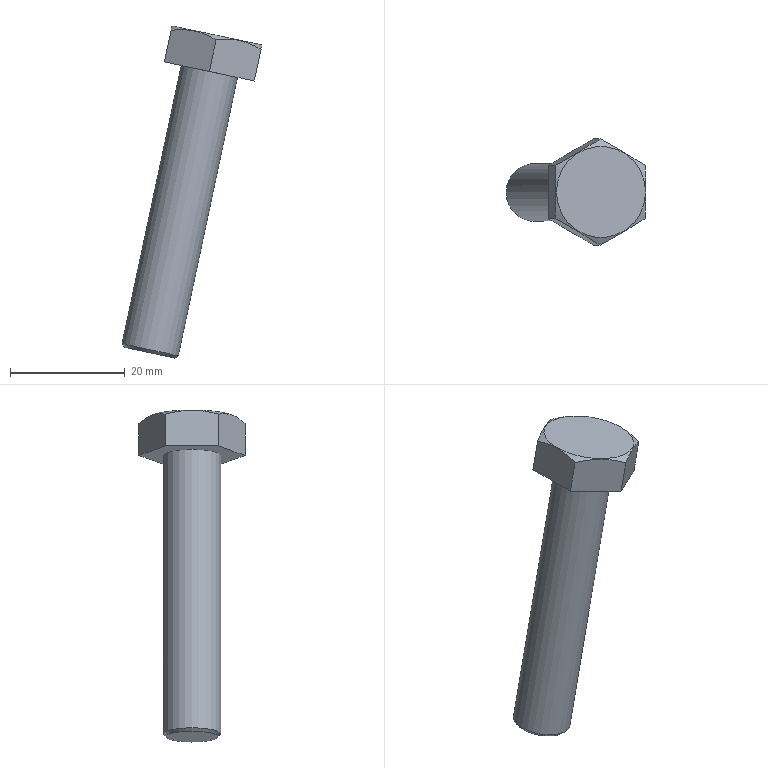Part | STEP file | 8901-M1050B (bolt M12×50) | 1 solid | 12 faces | box 24.329 x 18.475 x 57.75 mm | volume 5337 mm3 | plane 9 | cone 2 | cylinder 1 | commonest cylinder face diameters 10 x1
STEP:
#1=CARTESIAN_POINT('',(0.,0.,0.));
#2=DIRECTION('',(0.,0.,1.));
#3=DIRECTION('',(1.,0.,0.));
#4=AXIS2_PLACEMENT_3D('',#1,#2,#3);
#5=CARTESIAN_POINT('',(1860.531,-39.5,-396.681));
#6=VERTEX_POINT('',#5);
#7=CARTESIAN_POINT('',(1865.421,-39.5,-397.721));
#8=DIRECTION('',(0.2079,0.,0.9781));
#9=DIRECTION('',(-0.9781,0.,0.2079));
#10=AXIS2_PLACEMENT_3D('',#7,#8,#9);
#11=CIRCLE('',#10,5.);
#12=CARTESIAN_POINT('',(1865.421,-39.5,-397.721));
#13=DIRECTION('',(0.2079,0.,0.9781));
#14=DIRECTION('',(-0.9781,0.,0.2079));
#15=AXIS2_PLACEMENT_3D('',#12,#13,#14);
#16=CONICAL_SURFACE('',#15,5.,0.7854);
#17=CARTESIAN_POINT('',(0.,0.));
#18=DIRECTION('',(1.,0.));
#19=VECTOR('',#18,1.);
#20=LINE('',#17,#19);
#21=(GEOMETRIC_REPRESENTATION_CONTEXT(2)PARAMETRIC_REPRESENTATION_CONTEXT()REPRESENTATION_CONTEXT('',''));
#22=DEFINITIONAL_REPRESENTATION('',(#20),#21);
#23=PCURVE('',#16,#22);
#24=CARTESIAN_POINT('',(1875.713,-39.5,-349.303));
#25=DIRECTION('',(-0.2079,0.,-0.9781));
#26=DIRECTION('',(0.9781,0.,-0.2079));
#27=AXIS2_PLACEMENT_3D('',#24,#25,#26);
#28=CYLINDRICAL_SURFACE('',#27,5.);
#29=CARTESIAN_POINT('',(9.425,49.5));
#30=DIRECTION('',(-1.,0.));
#31=VECTOR('',#30,1.);
#32=LINE('',#29,#31);
#33=(GEOMETRIC_REPRESENTATION_CONTEXT(2)PARAMETRIC_REPRESENTATION_CONTEXT()REPRESENTATION_CONTEXT('',''));
#34=DEFINITIONAL_REPRESENTATION('',(#32),#33);
#35=PCURVE('',#28,#34);
#36=SURFACE_CURVE('',#11,(#23,#35),.PCURVE_S1.);
#37=EDGE_CURVE('',#6,#6,#36,.T.);
#38=ORIENTED_EDGE('',*,*,#37,.F.);
#39=CARTESIAN_POINT('',(1860.916,-39.5,-397.274));
#40=VERTEX_POINT('',#39);
#41=CARTESIAN_POINT('',(1860.916,-39.5,-397.274));
#42=CARTESIAN_POINT('',(1860.531,-39.5,-396.681));
#43=B_SPLINE_CURVE_WITH_KNOTS('',1,(#41,#42),.UNSPECIFIED.,.F.,.F.,(2,2),(-0.7071,0.),.PIECEWISE_BEZIER_KNOTS.);
#44=CARTESIAN_POINT('',(0.,0.));
#45=DIRECTION('',(0.,1.));
#46=VECTOR('',#45,1.);
#47=LINE('',#44,#46);
#48=(GEOMETRIC_REPRESENTATION_CONTEXT(2)PARAMETRIC_REPRESENTATION_CONTEXT()REPRESENTATION_CONTEXT('',''));
#49=DEFINITIONAL_REPRESENTATION('',(#47),#48);
#50=PCURVE('',#16,#49);
#51=CARTESIAN_POINT('',(6.283,0.));
#52=DIRECTION('',(0.,1.));
#53=VECTOR('',#52,1.);
#54=LINE('',#51,#53);
#55=(GEOMETRIC_REPRESENTATION_CONTEXT(2)PARAMETRIC_REPRESENTATION_CONTEXT()REPRESENTATION_CONTEXT('',''));
#56=DEFINITIONAL_REPRESENTATION('',(#54),#55);
#57=PCURVE('',#16,#56);
#58=SEAM_CURVE('',#43,(#50,#57),.PCURVE_S1.);
#59=EDGE_CURVE('',#40,#6,#58,.T.);
#60=ORIENTED_EDGE('',*,*,#59,.F.);
#61=CARTESIAN_POINT('',(1865.317,-39.5,-398.21));
#62=DIRECTION('',(-0.2079,0.,-0.9781));
#63=DIRECTION('',(-0.9781,0.,0.2079));
#64=AXIS2_PLACEMENT_3D('',#61,#62,#63);
#65=CIRCLE('',#64,4.5);
#66=CARTESIAN_POINT('',(6.283,-0.5));
#67=DIRECTION('',(-1.,0.));
#68=VECTOR('',#67,1.);
#69=LINE('',#66,#68);
#70=(GEOMETRIC_REPRESENTATION_CONTEXT(2)PARAMETRIC_REPRESENTATION_CONTEXT()REPRESENTATION_CONTEXT('',''));
#71=DEFINITIONAL_REPRESENTATION('',(#69),#70);
#72=PCURVE('',#16,#71);
#73=CARTESIAN_POINT('',(1865.317,-39.5,-398.21));
#74=DIRECTION('',(-0.2079,0.,-0.9781));
#75=DIRECTION('',(0.9781,0.,-0.2079));
#76=AXIS2_PLACEMENT_3D('',#73,#74,#75);
#77=PLANE('',#76);
#78=CARTESIAN_POINT('',(0.,0.));
#79=DIRECTION('',(-1.,0.));
#80=AXIS2_PLACEMENT_2D('',#78,#79);
#81=CIRCLE('',#80,4.5);
#82=(GEOMETRIC_REPRESENTATION_CONTEXT(2)PARAMETRIC_REPRESENTATION_CONTEXT()REPRESENTATION_CONTEXT('',''));
#83=DEFINITIONAL_REPRESENTATION('',(#81),#82);
#84=PCURVE('',#77,#83);
#85=SURFACE_CURVE('',#65,(#72,#84),.PCURVE_S1.);
#86=EDGE_CURVE('',#40,#40,#85,.T.);
#87=ORIENTED_EDGE('',*,*,#86,.F.);
#88=ORIENTED_EDGE('',*,*,#59,.T.);
#89=EDGE_LOOP('',(#38,#60,#87,#88));
#90=FACE_BOUND('',#89,.T.);
#91=ADVANCED_FACE('',(#90),#16,.T.);
#92=ORIENTED_EDGE('',*,*,#86,.T.);
#93=EDGE_LOOP('',(#92));
#94=FACE_BOUND('',#93,.T.);
#95=ADVANCED_FACE('',(#94),#77,.T.);
#96=CARTESIAN_POINT('',(1884.791,-39.5,-344.689));
#97=VERTEX_POINT('',#96);
#98=CARTESIAN_POINT('',(1877.044,-39.5,-343.043));
#99=DIRECTION('',(0.2079,0.,0.9781));
#100=DIRECTION('',(0.9781,0.,-0.2079));
#101=AXIS2_PLACEMENT_3D('',#98,#99,#100);
#102=CIRCLE('',#101,7.92);
#103=CARTESIAN_POINT('',(1877.044,-39.5,-343.043));
#104=DIRECTION('',(0.2079,0.,0.9781));
#105=DIRECTION('',(-0.9781,0.,0.2079));
#106=AXIS2_PLACEMENT_3D('',#103,#104,#105);
#107=PLANE('',#106);
#108=CARTESIAN_POINT('',(0.,0.));
#109=DIRECTION('',(-1.,0.));
#110=AXIS2_PLACEMENT_2D('',#108,#109);
#111=CIRCLE('',#110,7.92);
#112=(GEOMETRIC_REPRESENTATION_CONTEXT(2)PARAMETRIC_REPRESENTATION_CONTEXT()REPRESENTATION_CONTEXT('',''));
#113=DEFINITIONAL_REPRESENTATION('',(#111),#112);
#114=PCURVE('',#107,#113);
#115=CARTESIAN_POINT('',(1877.994,-39.5,-338.57));
#116=DIRECTION('',(-0.2079,0.,-0.9781));
#117=DIRECTION('',(0.9781,0.,-0.2079));
#118=AXIS2_PLACEMENT_3D('',#115,#116,#117);
#119=CONICAL_SURFACE('',#118,0.,1.047);
#120=CARTESIAN_POINT('',(6.283,4.573));
#121=DIRECTION('',(-1.,0.));
#122=VECTOR('',#121,1.);
#123=LINE('',#120,#122);
#124=(GEOMETRIC_REPRESENTATION_CONTEXT(2)PARAMETRIC_REPRESENTATION_CONTEXT()REPRESENTATION_CONTEXT('',''));
#125=DEFINITIONAL_REPRESENTATION('',(#123),#124);
#126=PCURVE('',#119,#125);
#127=SURFACE_CURVE('',#102,(#114,#126),.PCURVE_S1.);
#128=EDGE_CURVE('',#97,#97,#127,.T.);
#129=ORIENTED_EDGE('',*,*,#128,.T.);
#130=EDGE_LOOP('',(#129));
#131=FACE_BOUND('',#130,.T.);
#132=ADVANCED_FACE('',(#131),#107,.T.);
#133=ORIENTED_EDGE('',*,*,#128,.F.);
#134=CARTESIAN_POINT('',(1884.859,-39.5,-344.751));
#135=VERTEX_POINT('',#134);
#136=CARTESIAN_POINT('',(1884.791,-39.5,-344.689));
#137=CARTESIAN_POINT('',(1884.859,-39.5,-344.751));
#138=B_SPLINE_CURVE_WITH_KNOTS('',1,(#136,#137),.UNSPECIFIED.,.F.,.F.,(2,2),(9.145,9.238),.PIECEWISE_BEZIER_KNOTS.);
#139=CARTESIAN_POINT('',(6.283,0.));
#140=DIRECTION('',(0.,1.));
#141=VECTOR('',#140,1.);
#142=LINE('',#139,#141);
#143=(GEOMETRIC_REPRESENTATION_CONTEXT(2)PARAMETRIC_REPRESENTATION_CONTEXT()REPRESENTATION_CONTEXT('',''));
#144=DEFINITIONAL_REPRESENTATION('',(#142),#143);
#145=PCURVE('',#119,#144);
#146=CARTESIAN_POINT('',(0.,0.));
#147=DIRECTION('',(0.,1.));
#148=VECTOR('',#147,1.);
#149=LINE('',#146,#148);
#150=(GEOMETRIC_REPRESENTATION_CONTEXT(2)PARAMETRIC_REPRESENTATION_CONTEXT()REPRESENTATION_CONTEXT('',''));
#151=DEFINITIONAL_REPRESENTATION('',(#149),#150);
#152=PCURVE('',#119,#151);
#153=SEAM_CURVE('',#138,(#145,#152),.PCURVE_S1.);
#154=EDGE_CURVE('',#97,#135,#153,.T.);
#155=ORIENTED_EDGE('',*,*,#154,.T.);
#156=CARTESIAN_POINT('',(1884.711,-34.881,-345.45));
#157=VERTEX_POINT('',#156);
#158=CARTESIAN_POINT('',(1884.711,-34.881,-345.45));
#159=CARTESIAN_POINT('',(1884.801,-36.389,-345.024));
#160=CARTESIAN_POINT('',(1884.859,-37.92,-344.752));
#161=CARTESIAN_POINT('',(1884.859,-41.062,-344.75));
#162=CARTESIAN_POINT('',(1884.801,-42.609,-345.023));
#163=CARTESIAN_POINT('',(1884.711,-44.119,-345.45));
#164=B_SPLINE_CURVE_WITH_KNOTS('',3,(#158,#159,#160,#161,#162,#163),.UNSPECIFIED.,.F.,.F.,(4,2,4),(0.,0.5,1.),.UNSPECIFIED.);
#165=CARTESIAN_POINT('',(5.76,5.333));
#166=CARTESIAN_POINT('',(5.772,5.294));
#167=CARTESIAN_POINT('',(5.799,5.217));
#168=CARTESIAN_POINT('',(5.84,5.11));
#169=CARTESIAN_POINT('',(5.883,5.013));
#170=CARTESIAN_POINT('',(5.928,4.924));
#171=CARTESIAN_POINT('',(5.975,4.846));
#172=CARTESIAN_POINT('',(6.023,4.778));
#173=CARTESIAN_POINT('',(6.073,4.721));
#174=CARTESIAN_POINT('',(6.124,4.676));
#175=CARTESIAN_POINT('',(6.176,4.644));
#176=CARTESIAN_POINT('',(6.229,4.624));
#177=CARTESIAN_POINT('',(6.282,4.617));
#178=CARTESIAN_POINT('',(6.336,4.623));
#179=CARTESIAN_POINT('',(6.389,4.643));
#180=CARTESIAN_POINT('',(6.441,4.675));
#181=CARTESIAN_POINT('',(6.492,4.72));
#182=CARTESIAN_POINT('',(6.542,4.776));
#183=CARTESIAN_POINT('',(6.591,4.844));
#184=CARTESIAN_POINT('',(6.638,4.923));
#185=CARTESIAN_POINT('',(6.683,5.012));
#186=CARTESIAN_POINT('',(6.726,5.11));
#187=CARTESIAN_POINT('',(6.768,5.217));
#188=CARTESIAN_POINT('',(6.794,5.294));
#189=CARTESIAN_POINT('',(6.807,5.333));
#190=B_SPLINE_CURVE_WITH_KNOTS('',3,(#165,#166,#167,#168,#169,#170,#171,#172,#173,#174,#175,#176,#177,#178,#179,#180,#181,#182,#183,#184,#185,#186,#187,#188,#189),.UNSPECIFIED.,.F.,.F.,(4,1,1,1,1,1,1,1,1,1,1,1,1,1,1,1,1,1,1,1,1,1,4),(0.,0.04545,0.09091,0.1364,0.1818,0.2273,0.2727,0.3182,0.3636,0.4091,0.4545,0.5,0.5455,0.5909,0.6364,0.6818,0.7273,0.7727,0.8182,0.8636,0.9091,0.9545,1.),.QUASI_UNIFORM_KNOTS.);
#191=(GEOMETRIC_REPRESENTATION_CONTEXT(2)PARAMETRIC_REPRESENTATION_CONTEXT()REPRESENTATION_CONTEXT('',''));
#192=DEFINITIONAL_REPRESENTATION('',(#190),#191);
#193=PCURVE('',#119,#192);
#194=CARTESIAN_POINT('',(1884.203,-39.5,-347.836));
#195=DIRECTION('',(0.9781,0.,-0.2079));
#196=DIRECTION('',(0.,-1.,0.));
#197=AXIS2_PLACEMENT_3D('',#194,#195,#196);
#198=PLANE('',#197);
#199=CARTESIAN_POINT('',(-4.619,-2.439));
#200=CARTESIAN_POINT('',(-3.11,-2.875));
#201=CARTESIAN_POINT('',(-1.58,-3.153));
#202=CARTESIAN_POINT('',(1.562,-3.155));
#203=CARTESIAN_POINT('',(3.109,-2.875));
#204=CARTESIAN_POINT('',(4.619,-2.439));
#205=B_SPLINE_CURVE_WITH_KNOTS('',3,(#199,#200,#201,#202,#203,#204),.UNSPECIFIED.,.F.,.F.,(4,2,4),(0.,0.5,1.),.UNSPECIFIED.);
#206=(GEOMETRIC_REPRESENTATION_CONTEXT(2)PARAMETRIC_REPRESENTATION_CONTEXT()REPRESENTATION_CONTEXT('',''));
#207=DEFINITIONAL_REPRESENTATION('',(#205),#206);
#208=PCURVE('',#198,#207);
#209=SURFACE_CURVE('',#164,(#193,#208),.PCURVE_S1.);
#210=EDGE_CURVE('',#157,#135,#209,.T.);
#211=ORIENTED_EDGE('',*,*,#210,.F.);
#212=CARTESIAN_POINT('',(1876.885,-30.262,-343.787));
#213=VERTEX_POINT('',#212);
#214=CARTESIAN_POINT('',(1876.885,-30.262,-343.787));
#215=CARTESIAN_POINT('',(1878.254,-31.017,-343.632));
#216=CARTESIAN_POINT('',(1879.608,-31.782,-343.636));
#217=CARTESIAN_POINT('',(1882.27,-33.353,-344.2));
#218=CARTESIAN_POINT('',(1883.522,-34.126,-344.752));
#219=CARTESIAN_POINT('',(1884.711,-34.881,-345.45));
#220=B_SPLINE_CURVE_WITH_KNOTS('',3,(#214,#215,#216,#217,#218,#219),.UNSPECIFIED.,.F.,.F.,(4,2,4),(0.,0.5,1.),.UNSPECIFIED.);
#221=CARTESIAN_POINT('',(4.712,5.333));
#222=CARTESIAN_POINT('',(4.725,5.294));
#223=CARTESIAN_POINT('',(4.752,5.217));
#224=CARTESIAN_POINT('',(4.793,5.11));
#225=CARTESIAN_POINT('',(4.836,5.013));
#226=CARTESIAN_POINT('',(4.881,4.924));
#227=CARTESIAN_POINT('',(4.928,4.846));
#228=CARTESIAN_POINT('',(4.976,4.778));
#229=CARTESIAN_POINT('',(5.026,4.721));
#230=CARTESIAN_POINT('',(5.076,4.676));
#231=CARTESIAN_POINT('',(5.129,4.644));
#232=CARTESIAN_POINT('',(5.181,4.624));
#233=CARTESIAN_POINT('',(5.235,4.617));
#234=CARTESIAN_POINT('',(5.288,4.623));
#235=CARTESIAN_POINT('',(5.341,4.643));
#236=CARTESIAN_POINT('',(5.394,4.675));
#237=CARTESIAN_POINT('',(5.445,4.72));
#238=CARTESIAN_POINT('',(5.495,4.776));
#239=CARTESIAN_POINT('',(5.543,4.844));
#240=CARTESIAN_POINT('',(5.59,4.923));
#241=CARTESIAN_POINT('',(5.636,5.012));
#242=CARTESIAN_POINT('',(5.679,5.11));
#243=CARTESIAN_POINT('',(5.72,5.217));
#244=CARTESIAN_POINT('',(5.747,5.294));
#245=CARTESIAN_POINT('',(5.76,5.333));
#246=B_SPLINE_CURVE_WITH_KNOTS('',3,(#221,#222,#223,#224,#225,#226,#227,#228,#229,#230,#231,#232,#233,#234,#235,#236,#237,#238,#239,#240,#241,#242,#243,#244,#245),.UNSPECIFIED.,.F.,.F.,(4,1,1,1,1,1,1,1,1,1,1,1,1,1,1,1,1,1,1,1,1,1,4),(0.,0.04545,0.09091,0.1364,0.1818,0.2273,0.2727,0.3182,0.3636,0.4091,0.4545,0.5,0.5455,0.5909,0.6364,0.6818,0.7273,0.7727,0.8182,0.8636,0.9091,0.9545,1.),.QUASI_UNIFORM_KNOTS.);
#247=(GEOMETRIC_REPRESENTATION_CONTEXT(2)PARAMETRIC_REPRESENTATION_CONTEXT()REPRESENTATION_CONTEXT('',''));
#248=DEFINITIONAL_REPRESENTATION('',(#246),#247);
#249=PCURVE('',#119,#248);
#250=CARTESIAN_POINT('',(1880.291,-32.572,-347.004));
#251=DIRECTION('',(0.4891,0.866,-0.104));
#252=DIRECTION('',(0.8471,-0.5,-0.1801));
#253=AXIS2_PLACEMENT_3D('',#250,#251,#252);
#254=PLANE('',#253);
#255=CARTESIAN_POINT('',(-4.619,-2.439));
#256=CARTESIAN_POINT('',(-3.11,-2.875));
#257=CARTESIAN_POINT('',(-1.58,-3.153));
#258=CARTESIAN_POINT('',(1.562,-3.155));
#259=CARTESIAN_POINT('',(3.109,-2.875));
#260=CARTESIAN_POINT('',(4.619,-2.439));
#261=B_SPLINE_CURVE_WITH_KNOTS('',3,(#255,#256,#257,#258,#259,#260),.UNSPECIFIED.,.F.,.F.,(4,2,4),(0.,0.5,1.),.UNSPECIFIED.);
#262=(GEOMETRIC_REPRESENTATION_CONTEXT(2)PARAMETRIC_REPRESENTATION_CONTEXT()REPRESENTATION_CONTEXT('',''));
#263=DEFINITIONAL_REPRESENTATION('',(#261),#262);
#264=PCURVE('',#254,#263);
#265=SURFACE_CURVE('',#220,(#249,#264),.PCURVE_S1.);
#266=EDGE_CURVE('',#213,#157,#265,.T.);
#267=ORIENTED_EDGE('',*,*,#266,.F.);
#268=CARTESIAN_POINT('',(1869.06,-34.881,-342.123));
#269=VERTEX_POINT('',#268);
#270=CARTESIAN_POINT('',(1869.06,-34.881,-342.123));
#271=CARTESIAN_POINT('',(1870.428,-34.127,-341.969));
#272=CARTESIAN_POINT('',(1871.783,-33.362,-341.973));
#273=CARTESIAN_POINT('',(1874.445,-31.791,-342.536));
#274=CARTESIAN_POINT('',(1875.697,-31.017,-343.088));
#275=CARTESIAN_POINT('',(1876.885,-30.262,-343.787));
#276=B_SPLINE_CURVE_WITH_KNOTS('',3,(#270,#271,#272,#273,#274,#275),.UNSPECIFIED.,.F.,.F.,(4,2,4),(0.,0.5,1.),.UNSPECIFIED.);
#277=CARTESIAN_POINT('',(3.665,5.333));
#278=CARTESIAN_POINT('',(3.678,5.294));
#279=CARTESIAN_POINT('',(3.704,5.217));
#280=CARTESIAN_POINT('',(3.746,5.11));
#281=CARTESIAN_POINT('',(3.789,5.013));
#282=CARTESIAN_POINT('',(3.834,4.924));
#283=CARTESIAN_POINT('',(3.88,4.846));
#284=CARTESIAN_POINT('',(3.929,4.778));
#285=CARTESIAN_POINT('',(3.978,4.721));
#286=CARTESIAN_POINT('',(4.029,4.676));
#287=CARTESIAN_POINT('',(4.081,4.644));
#288=CARTESIAN_POINT('',(4.134,4.624));
#289=CARTESIAN_POINT('',(4.188,4.617));
#290=CARTESIAN_POINT('',(4.241,4.623));
#291=CARTESIAN_POINT('',(4.294,4.643));
#292=CARTESIAN_POINT('',(4.346,4.675));
#293=CARTESIAN_POINT('',(4.398,4.72));
#294=CARTESIAN_POINT('',(4.448,4.776));
#295=CARTESIAN_POINT('',(4.496,4.844));
#296=CARTESIAN_POINT('',(4.543,4.923));
#297=CARTESIAN_POINT('',(4.588,5.012));
#298=CARTESIAN_POINT('',(4.632,5.11));
#299=CARTESIAN_POINT('',(4.673,5.217));
#300=CARTESIAN_POINT('',(4.7,5.294));
#301=CARTESIAN_POINT('',(4.712,5.333));
#302=B_SPLINE_CURVE_WITH_KNOTS('',3,(#277,#278,#279,#280,#281,#282,#283,#284,#285,#286,#287,#288,#289,#290,#291,#292,#293,#294,#295,#296,#297,#298,#299,#300,#301),.UNSPECIFIED.,.F.,.F.,(4,1,1,1,1,1,1,1,1,1,1,1,1,1,1,1,1,1,1,1,1,1,4),(0.,0.04545,0.09091,0.1364,0.1818,0.2273,0.2727,0.3182,0.3636,0.4091,0.4545,0.5,0.5455,0.5909,0.6364,0.6818,0.7273,0.7727,0.8182,0.8636,0.9091,0.9545,1.),.QUASI_UNIFORM_KNOTS.);
#303=(GEOMETRIC_REPRESENTATION_CONTEXT(2)PARAMETRIC_REPRESENTATION_CONTEXT()REPRESENTATION_CONTEXT('',''));
#304=DEFINITIONAL_REPRESENTATION('',(#302),#303);
#305=PCURVE('',#119,#304);
#306=CARTESIAN_POINT('',(1872.466,-32.572,-345.341));
#307=DIRECTION('',(-0.4891,0.866,0.104));
#308=DIRECTION('',(0.8471,0.5,-0.1801));
#309=AXIS2_PLACEMENT_3D('',#306,#307,#308);
#310=PLANE('',#309);
#311=CARTESIAN_POINT('',(-4.619,-2.439));
#312=CARTESIAN_POINT('',(-3.11,-2.875));
#313=CARTESIAN_POINT('',(-1.58,-3.153));
#314=CARTESIAN_POINT('',(1.562,-3.155));
#315=CARTESIAN_POINT('',(3.109,-2.875));
#316=CARTESIAN_POINT('',(4.619,-2.439));
#317=B_SPLINE_CURVE_WITH_KNOTS('',3,(#311,#312,#313,#314,#315,#316),.UNSPECIFIED.,.F.,.F.,(4,2,4),(0.,0.5,1.),.UNSPECIFIED.);
#318=(GEOMETRIC_REPRESENTATION_CONTEXT(2)PARAMETRIC_REPRESENTATION_CONTEXT()REPRESENTATION_CONTEXT('',''));
#319=DEFINITIONAL_REPRESENTATION('',(#317),#318);
#320=PCURVE('',#310,#319);
#321=SURFACE_CURVE('',#276,(#305,#320),.PCURVE_S1.);
#322=EDGE_CURVE('',#269,#213,#321,.T.);
#323=ORIENTED_EDGE('',*,*,#322,.F.);
#324=CARTESIAN_POINT('',(1869.06,-44.119,-342.123));
#325=VERTEX_POINT('',#324);
#326=CARTESIAN_POINT('',(1869.06,-44.119,-342.123));
#327=CARTESIAN_POINT('',(1869.151,-42.61,-341.697));
#328=CARTESIAN_POINT('',(1869.209,-41.08,-341.425));
#329=CARTESIAN_POINT('',(1869.209,-37.938,-341.423));
#330=CARTESIAN_POINT('',(1869.151,-36.391,-341.697));
#331=CARTESIAN_POINT('',(1869.06,-34.881,-342.123));
#332=B_SPLINE_CURVE_WITH_KNOTS('',3,(#326,#327,#328,#329,#330,#331),.UNSPECIFIED.,.F.,.F.,(4,2,4),(0.,0.5,1.),.UNSPECIFIED.);
#333=CARTESIAN_POINT('',(2.618,5.333));
#334=CARTESIAN_POINT('',(2.631,5.294));
#335=CARTESIAN_POINT('',(2.657,5.217));
#336=CARTESIAN_POINT('',(2.698,5.11));
#337=CARTESIAN_POINT('',(2.742,5.013));
#338=CARTESIAN_POINT('',(2.787,4.924));
#339=CARTESIAN_POINT('',(2.833,4.846));
#340=CARTESIAN_POINT('',(2.881,4.778));
#341=CARTESIAN_POINT('',(2.931,4.721));
#342=CARTESIAN_POINT('',(2.982,4.676));
#343=CARTESIAN_POINT('',(3.034,4.644));
#344=CARTESIAN_POINT('',(3.087,4.624));
#345=CARTESIAN_POINT('',(3.14,4.617));
#346=CARTESIAN_POINT('',(3.194,4.623));
#347=CARTESIAN_POINT('',(3.247,4.643));
#348=CARTESIAN_POINT('',(3.299,4.675));
#349=CARTESIAN_POINT('',(3.351,4.72));
#350=CARTESIAN_POINT('',(3.401,4.776));
#351=CARTESIAN_POINT('',(3.449,4.844));
#352=CARTESIAN_POINT('',(3.496,4.923));
#353=CARTESIAN_POINT('',(3.541,5.012));
#354=CARTESIAN_POINT('',(3.584,5.11));
#355=CARTESIAN_POINT('',(3.626,5.217));
#356=CARTESIAN_POINT('',(3.652,5.294));
#357=CARTESIAN_POINT('',(3.665,5.333));
#358=B_SPLINE_CURVE_WITH_KNOTS('',3,(#333,#334,#335,#336,#337,#338,#339,#340,#341,#342,#343,#344,#345,#346,#347,#348,#349,#350,#351,#352,#353,#354,#355,#356,#357),.UNSPECIFIED.,.F.,.F.,(4,1,1,1,1,1,1,1,1,1,1,1,1,1,1,1,1,1,1,1,1,1,4),(0.,0.04545,0.09091,0.1364,0.1818,0.2273,0.2727,0.3182,0.3636,0.4091,0.4545,0.5,0.5455,0.5909,0.6364,0.6818,0.7273,0.7727,0.8182,0.8636,0.9091,0.9545,1.),.QUASI_UNIFORM_KNOTS.);
#359=(GEOMETRIC_REPRESENTATION_CONTEXT(2)PARAMETRIC_REPRESENTATION_CONTEXT()REPRESENTATION_CONTEXT('',''));
#360=DEFINITIONAL_REPRESENTATION('',(#358),#359);
#361=PCURVE('',#119,#360);
#362=CARTESIAN_POINT('',(1868.553,-39.5,-344.509));
#363=DIRECTION('',(-0.9781,0.,0.2079));
#364=DIRECTION('',(0.,1.,0.));
#365=AXIS2_PLACEMENT_3D('',#362,#363,#364);
#366=PLANE('',#365);
#367=CARTESIAN_POINT('',(-4.619,-2.439));
#368=CARTESIAN_POINT('',(-3.11,-2.875));
#369=CARTESIAN_POINT('',(-1.58,-3.153));
#370=CARTESIAN_POINT('',(1.562,-3.155));
#371=CARTESIAN_POINT('',(3.109,-2.875));
#372=CARTESIAN_POINT('',(4.619,-2.439));
#373=B_SPLINE_CURVE_WITH_KNOTS('',3,(#367,#368,#369,#370,#371,#372),.UNSPECIFIED.,.F.,.F.,(4,2,4),(0.,0.5,1.),.UNSPECIFIED.);
#374=(GEOMETRIC_REPRESENTATION_CONTEXT(2)PARAMETRIC_REPRESENTATION_CONTEXT()REPRESENTATION_CONTEXT('',''));
#375=DEFINITIONAL_REPRESENTATION('',(#373),#374);
#376=PCURVE('',#366,#375);
#377=SURFACE_CURVE('',#332,(#361,#376),.PCURVE_S1.);
#378=EDGE_CURVE('',#325,#269,#377,.T.);
#379=ORIENTED_EDGE('',*,*,#378,.F.);
#380=CARTESIAN_POINT('',(1876.885,-48.738,-343.787));
#381=VERTEX_POINT('',#380);
#382=CARTESIAN_POINT('',(1876.885,-48.738,-343.787));
#383=CARTESIAN_POINT('',(1875.698,-47.983,-343.089));
#384=CARTESIAN_POINT('',(1874.459,-47.218,-342.541));
#385=CARTESIAN_POINT('',(1871.799,-45.647,-341.974));
#386=CARTESIAN_POINT('',(1870.43,-44.874,-341.969));
#387=CARTESIAN_POINT('',(1869.06,-44.119,-342.123));
#388=B_SPLINE_CURVE_WITH_KNOTS('',3,(#382,#383,#384,#385,#386,#387),.UNSPECIFIED.,.F.,.F.,(4,2,4),(0.,0.5,1.),.UNSPECIFIED.);
#389=CARTESIAN_POINT('',(1.571,5.333));
#390=CARTESIAN_POINT('',(1.584,5.294));
#391=CARTESIAN_POINT('',(1.61,5.217));
#392=CARTESIAN_POINT('',(1.651,5.11));
#393=CARTESIAN_POINT('',(1.694,5.013));
#394=CARTESIAN_POINT('',(1.739,4.924));
#395=CARTESIAN_POINT('',(1.786,4.846));
#396=CARTESIAN_POINT('',(1.834,4.778));
#397=CARTESIAN_POINT('',(1.884,4.721));
#398=CARTESIAN_POINT('',(1.935,4.676));
#399=CARTESIAN_POINT('',(1.987,4.644));
#400=CARTESIAN_POINT('',(2.04,4.624));
#401=CARTESIAN_POINT('',(2.093,4.617));
#402=CARTESIAN_POINT('',(2.147,4.623));
#403=CARTESIAN_POINT('',(2.2,4.643));
#404=CARTESIAN_POINT('',(2.252,4.675));
#405=CARTESIAN_POINT('',(2.303,4.72));
#406=CARTESIAN_POINT('',(2.353,4.776));
#407=CARTESIAN_POINT('',(2.402,4.844));
#408=CARTESIAN_POINT('',(2.449,4.923));
#409=CARTESIAN_POINT('',(2.494,5.012));
#410=CARTESIAN_POINT('',(2.537,5.11));
#411=CARTESIAN_POINT('',(2.579,5.217));
#412=CARTESIAN_POINT('',(2.605,5.294));
#413=CARTESIAN_POINT('',(2.618,5.333));
#414=B_SPLINE_CURVE_WITH_KNOTS('',3,(#389,#390,#391,#392,#393,#394,#395,#396,#397,#398,#399,#400,#401,#402,#403,#404,#405,#406,#407,#408,#409,#410,#411,#412,#413),.UNSPECIFIED.,.F.,.F.,(4,1,1,1,1,1,1,1,1,1,1,1,1,1,1,1,1,1,1,1,1,1,4),(0.,0.04545,0.09091,0.1364,0.1818,0.2273,0.2727,0.3182,0.3636,0.4091,0.4545,0.5,0.5455,0.5909,0.6364,0.6818,0.7273,0.7727,0.8182,0.8636,0.9091,0.9545,1.),.QUASI_UNIFORM_KNOTS.);
#415=(GEOMETRIC_REPRESENTATION_CONTEXT(2)PARAMETRIC_REPRESENTATION_CONTEXT()REPRESENTATION_CONTEXT('',''));
#416=DEFINITIONAL_REPRESENTATION('',(#414),#415);
#417=PCURVE('',#119,#416);
#418=CARTESIAN_POINT('',(1872.466,-46.428,-345.341));
#419=DIRECTION('',(-0.4891,-0.866,0.104));
#420=DIRECTION('',(-0.8471,0.5,0.1801));
#421=AXIS2_PLACEMENT_3D('',#418,#419,#420);
#422=PLANE('',#421);
#423=CARTESIAN_POINT('',(-4.619,-2.439));
#424=CARTESIAN_POINT('',(-3.11,-2.875));
#425=CARTESIAN_POINT('',(-1.58,-3.153));
#426=CARTESIAN_POINT('',(1.562,-3.155));
#427=CARTESIAN_POINT('',(3.109,-2.875));
#428=CARTESIAN_POINT('',(4.619,-2.439));
#429=B_SPLINE_CURVE_WITH_KNOTS('',3,(#423,#424,#425,#426,#427,#428),.UNSPECIFIED.,.F.,.F.,(4,2,4),(0.,0.5,1.),.UNSPECIFIED.);
#430=(GEOMETRIC_REPRESENTATION_CONTEXT(2)PARAMETRIC_REPRESENTATION_CONTEXT()REPRESENTATION_CONTEXT('',''));
#431=DEFINITIONAL_REPRESENTATION('',(#429),#430);
#432=PCURVE('',#422,#431);
#433=SURFACE_CURVE('',#388,(#417,#432),.PCURVE_S1.);
#434=EDGE_CURVE('',#381,#325,#433,.T.);
#435=ORIENTED_EDGE('',*,*,#434,.F.);
#436=CARTESIAN_POINT('',(1884.711,-44.119,-345.45));
#437=VERTEX_POINT('',#436);
#438=CARTESIAN_POINT('',(1884.711,-44.119,-345.45));
#439=CARTESIAN_POINT('',(1883.523,-44.873,-344.752));
#440=CARTESIAN_POINT('',(1882.284,-45.638,-344.205));
#441=CARTESIAN_POINT('',(1879.624,-47.209,-343.637));
#442=CARTESIAN_POINT('',(1878.255,-47.982,-343.632));
#443=CARTESIAN_POINT('',(1876.885,-48.738,-343.787));
#444=B_SPLINE_CURVE_WITH_KNOTS('',3,(#438,#439,#440,#441,#442,#443),.UNSPECIFIED.,.F.,.F.,(4,2,4),(0.,0.5,1.),.UNSPECIFIED.);
#445=CARTESIAN_POINT('',(0.5236,5.333));
#446=CARTESIAN_POINT('',(0.5365,5.294));
#447=CARTESIAN_POINT('',(0.5628,5.217));
#448=CARTESIAN_POINT('',(0.6041,5.11));
#449=CARTESIAN_POINT('',(0.6472,5.013));
#450=CARTESIAN_POINT('',(0.6921,4.924));
#451=CARTESIAN_POINT('',(0.7388,4.846));
#452=CARTESIAN_POINT('',(0.787,4.778));
#453=CARTESIAN_POINT('',(0.8367,4.721));
#454=CARTESIAN_POINT('',(0.8877,4.676));
#455=CARTESIAN_POINT('',(0.9398,4.644));
#456=CARTESIAN_POINT('',(0.9926,4.624));
#457=CARTESIAN_POINT('',(1.046,4.617));
#458=CARTESIAN_POINT('',(1.1,4.623));
#459=CARTESIAN_POINT('',(1.153,4.643));
#460=CARTESIAN_POINT('',(1.205,4.675));
#461=CARTESIAN_POINT('',(1.256,4.72));
#462=CARTESIAN_POINT('',(1.306,4.776));
#463=CARTESIAN_POINT('',(1.355,4.844));
#464=CARTESIAN_POINT('',(1.402,4.923));
#465=CARTESIAN_POINT('',(1.447,5.012));
#466=CARTESIAN_POINT('',(1.49,5.11));
#467=CARTESIAN_POINT('',(1.532,5.217));
#468=CARTESIAN_POINT('',(1.558,5.294));
#469=CARTESIAN_POINT('',(1.571,5.333));
#470=B_SPLINE_CURVE_WITH_KNOTS('',3,(#445,#446,#447,#448,#449,#450,#451,#452,#453,#454,#455,#456,#457,#458,#459,#460,#461,#462,#463,#464,#465,#466,#467,#468,#469),.UNSPECIFIED.,.F.,.F.,(4,1,1,1,1,1,1,1,1,1,1,1,1,1,1,1,1,1,1,1,1,1,4),(0.,0.04545,0.09091,0.1364,0.1818,0.2273,0.2727,0.3182,0.3636,0.4091,0.4545,0.5,0.5455,0.5909,0.6364,0.6818,0.7273,0.7727,0.8182,0.8636,0.9091,0.9545,1.),.QUASI_UNIFORM_KNOTS.);
#471=(GEOMETRIC_REPRESENTATION_CONTEXT(2)PARAMETRIC_REPRESENTATION_CONTEXT()REPRESENTATION_CONTEXT('',''));
#472=DEFINITIONAL_REPRESENTATION('',(#470),#471);
#473=PCURVE('',#119,#472);
#474=CARTESIAN_POINT('',(1880.291,-46.428,-347.004));
#475=DIRECTION('',(0.4891,-0.866,-0.104));
#476=DIRECTION('',(-0.8471,-0.5,0.1801));
#477=AXIS2_PLACEMENT_3D('',#474,#475,#476);
#478=PLANE('',#477);
#479=CARTESIAN_POINT('',(-4.619,-2.439));
#480=CARTESIAN_POINT('',(-3.11,-2.875));
#481=CARTESIAN_POINT('',(-1.58,-3.153));
#482=CARTESIAN_POINT('',(1.562,-3.155));
#483=CARTESIAN_POINT('',(3.109,-2.875));
#484=CARTESIAN_POINT('',(4.619,-2.439));
#485=B_SPLINE_CURVE_WITH_KNOTS('',3,(#479,#480,#481,#482,#483,#484),.UNSPECIFIED.,.F.,.F.,(4,2,4),(0.,0.5,1.),.UNSPECIFIED.);
#486=(GEOMETRIC_REPRESENTATION_CONTEXT(2)PARAMETRIC_REPRESENTATION_CONTEXT()REPRESENTATION_CONTEXT('',''));
#487=DEFINITIONAL_REPRESENTATION('',(#485),#486);
#488=PCURVE('',#478,#487);
#489=SURFACE_CURVE('',#444,(#473,#488),.PCURVE_S1.);
#490=EDGE_CURVE('',#437,#381,#489,.T.);
#491=ORIENTED_EDGE('',*,*,#490,.F.);
#492=CARTESIAN_POINT('',(1884.711,-34.881,-345.45));
#493=CARTESIAN_POINT('',(1884.801,-36.389,-345.024));
#494=CARTESIAN_POINT('',(1884.859,-37.92,-344.752));
#495=CARTESIAN_POINT('',(1884.859,-41.062,-344.75));
#496=CARTESIAN_POINT('',(1884.801,-42.609,-345.023));
#497=CARTESIAN_POINT('',(1884.711,-44.119,-345.45));
#498=B_SPLINE_CURVE_WITH_KNOTS('',3,(#492,#493,#494,#495,#496,#497),.UNSPECIFIED.,.F.,.F.,(4,2,4),(0.,0.5,1.),.UNSPECIFIED.);
#499=CARTESIAN_POINT('',(-0.5236,5.333));
#500=CARTESIAN_POINT('',(-0.5107,5.294));
#501=CARTESIAN_POINT('',(-0.4844,5.217));
#502=CARTESIAN_POINT('',(-0.4431,5.11));
#503=CARTESIAN_POINT('',(-0.4,5.013));
#504=CARTESIAN_POINT('',(-0.3551,4.924));
#505=CARTESIAN_POINT('',(-0.3084,4.846));
#506=CARTESIAN_POINT('',(-0.2602,4.778));
#507=CARTESIAN_POINT('',(-0.2105,4.721));
#508=CARTESIAN_POINT('',(-0.1595,4.676));
#509=CARTESIAN_POINT('',(-0.1074,4.644));
#510=CARTESIAN_POINT('',(-0.05458,4.624));
#511=CARTESIAN_POINT('',(-0.001113,4.617));
#512=CARTESIAN_POINT('',(0.0524,4.623));
#513=CARTESIAN_POINT('',(0.1054,4.643));
#514=CARTESIAN_POINT('',(0.1577,4.675));
#515=CARTESIAN_POINT('',(0.2089,4.72));
#516=CARTESIAN_POINT('',(0.2589,4.776));
#517=CARTESIAN_POINT('',(0.3075,4.844));
#518=CARTESIAN_POINT('',(0.3544,4.923));
#519=CARTESIAN_POINT('',(0.3996,5.012));
#520=CARTESIAN_POINT('',(0.4429,5.11));
#521=CARTESIAN_POINT('',(0.4844,5.217));
#522=CARTESIAN_POINT('',(0.5107,5.294));
#523=CARTESIAN_POINT('',(0.5236,5.333));
#524=B_SPLINE_CURVE_WITH_KNOTS('',3,(#499,#500,#501,#502,#503,#504,#505,#506,#507,#508,#509,#510,#511,#512,#513,#514,#515,#516,#517,#518,#519,#520,#521,#522,#523),.UNSPECIFIED.,.F.,.F.,(4,1,1,1,1,1,1,1,1,1,1,1,1,1,1,1,1,1,1,1,1,1,4),(0.,0.04545,0.09091,0.1364,0.1818,0.2273,0.2727,0.3182,0.3636,0.4091,0.4545,0.5,0.5455,0.5909,0.6364,0.6818,0.7273,0.7727,0.8182,0.8636,0.9091,0.9545,1.),.QUASI_UNIFORM_KNOTS.);
#525=(GEOMETRIC_REPRESENTATION_CONTEXT(2)PARAMETRIC_REPRESENTATION_CONTEXT()REPRESENTATION_CONTEXT('',''));
#526=DEFINITIONAL_REPRESENTATION('',(#524),#525);
#527=PCURVE('',#119,#526);
#528=CARTESIAN_POINT('',(-4.619,-2.439));
#529=CARTESIAN_POINT('',(-3.11,-2.875));
#530=CARTESIAN_POINT('',(-1.58,-3.153));
#531=CARTESIAN_POINT('',(1.562,-3.155));
#532=CARTESIAN_POINT('',(3.109,-2.875));
#533=CARTESIAN_POINT('',(4.619,-2.439));
#534=B_SPLINE_CURVE_WITH_KNOTS('',3,(#528,#529,#530,#531,#532,#533),.UNSPECIFIED.,.F.,.F.,(4,2,4),(0.,0.5,1.),.UNSPECIFIED.);
#535=(GEOMETRIC_REPRESENTATION_CONTEXT(2)PARAMETRIC_REPRESENTATION_CONTEXT()REPRESENTATION_CONTEXT('',''));
#536=DEFINITIONAL_REPRESENTATION('',(#534),#535);
#537=PCURVE('',#198,#536);
#538=SURFACE_CURVE('',#498,(#527,#537),.PCURVE_S1.);
#539=EDGE_CURVE('',#135,#437,#538,.T.);
#540=ORIENTED_EDGE('',*,*,#539,.F.);
#541=ORIENTED_EDGE('',*,*,#154,.F.);
#542=EDGE_LOOP('',(#133,#155,#211,#267,#323,#379,#435,#491,#540,#541));
#543=FACE_BOUND('',#542,.T.);
#544=ADVANCED_FACE('',(#543),#119,.T.);
#545=CARTESIAN_POINT('',(1875.713,-48.738,-349.303));
#546=VERTEX_POINT('',#545);
#547=CARTESIAN_POINT('',(1883.538,-44.119,-350.966));
#548=VERTEX_POINT('',#547);
#549=CARTESIAN_POINT('',(1875.713,-48.738,-349.303));
#550=DIRECTION('',(0.8471,0.5,-0.1801));
#551=VECTOR('',#550,1.);
#552=LINE('',#549,#551);
#553=CARTESIAN_POINT('',(1875.713,-39.5,-349.303));
#554=DIRECTION('',(-0.2079,0.,-0.9781));
#555=DIRECTION('',(0.9781,0.,-0.2079));
#556=AXIS2_PLACEMENT_3D('',#553,#554,#555);
#557=PLANE('',#556);
#558=CARTESIAN_POINT('',(0.,9.238));
#559=DIRECTION('',(0.866,-0.5));
#560=VECTOR('',#559,1.);
#561=LINE('',#558,#560);
#562=(GEOMETRIC_REPRESENTATION_CONTEXT(2)PARAMETRIC_REPRESENTATION_CONTEXT()REPRESENTATION_CONTEXT('',''));
#563=DEFINITIONAL_REPRESENTATION('',(#561),#562);
#564=PCURVE('',#557,#563);
#565=CARTESIAN_POINT('',(4.619,3.2));
#566=DIRECTION('',(-1.,0.));
#567=VECTOR('',#566,1.);
#568=LINE('',#565,#567);
#569=(GEOMETRIC_REPRESENTATION_CONTEXT(2)PARAMETRIC_REPRESENTATION_CONTEXT()REPRESENTATION_CONTEXT('',''));
#570=DEFINITIONAL_REPRESENTATION('',(#568),#569);
#571=PCURVE('',#478,#570);
#572=SURFACE_CURVE('',#552,(#564,#571),.PCURVE_S1.);
#573=EDGE_CURVE('',#546,#548,#572,.T.);
#574=ORIENTED_EDGE('',*,*,#573,.F.);
#575=CARTESIAN_POINT('',(1867.888,-44.119,-347.639));
#576=VERTEX_POINT('',#575);
#577=CARTESIAN_POINT('',(1867.888,-44.119,-347.639));
#578=DIRECTION('',(0.8471,-0.5,-0.1801));
#579=VECTOR('',#578,1.);
#580=LINE('',#577,#579);
#581=CARTESIAN_POINT('',(-8.,4.619));
#582=DIRECTION('',(0.866,0.5));
#583=VECTOR('',#582,1.);
#584=LINE('',#581,#583);
#585=(GEOMETRIC_REPRESENTATION_CONTEXT(2)PARAMETRIC_REPRESENTATION_CONTEXT()REPRESENTATION_CONTEXT('',''));
#586=DEFINITIONAL_REPRESENTATION('',(#584),#585);
#587=PCURVE('',#557,#586);
#588=CARTESIAN_POINT('',(4.619,3.2));
#589=DIRECTION('',(-1.,0.));
#590=VECTOR('',#589,1.);
#591=LINE('',#588,#590);
#592=(GEOMETRIC_REPRESENTATION_CONTEXT(2)PARAMETRIC_REPRESENTATION_CONTEXT()REPRESENTATION_CONTEXT('',''));
#593=DEFINITIONAL_REPRESENTATION('',(#591),#592);
#594=PCURVE('',#422,#593);
#595=SURFACE_CURVE('',#580,(#587,#594),.PCURVE_S1.);
#596=EDGE_CURVE('',#576,#546,#595,.T.);
#597=ORIENTED_EDGE('',*,*,#596,.F.);
#598=CARTESIAN_POINT('',(1867.888,-34.881,-347.639));
#599=VERTEX_POINT('',#598);
#600=CARTESIAN_POINT('',(1867.888,-34.881,-347.639));
#601=DIRECTION('',(0.,-1.,0.));
#602=VECTOR('',#601,1.);
#603=LINE('',#600,#602);
#604=CARTESIAN_POINT('',(-8.,-4.619));
#605=DIRECTION('',(0.,1.));
#606=VECTOR('',#605,1.);
#607=LINE('',#604,#606);
#608=(GEOMETRIC_REPRESENTATION_CONTEXT(2)PARAMETRIC_REPRESENTATION_CONTEXT()REPRESENTATION_CONTEXT('',''));
#609=DEFINITIONAL_REPRESENTATION('',(#607),#608);
#610=PCURVE('',#557,#609);
#611=CARTESIAN_POINT('',(4.619,3.2));
#612=DIRECTION('',(-1.,0.));
#613=VECTOR('',#612,1.);
#614=LINE('',#611,#613);
#615=(GEOMETRIC_REPRESENTATION_CONTEXT(2)PARAMETRIC_REPRESENTATION_CONTEXT()REPRESENTATION_CONTEXT('',''));
#616=DEFINITIONAL_REPRESENTATION('',(#614),#615);
#617=PCURVE('',#366,#616);
#618=SURFACE_CURVE('',#603,(#610,#617),.PCURVE_S1.);
#619=EDGE_CURVE('',#599,#576,#618,.T.);
#620=ORIENTED_EDGE('',*,*,#619,.F.);
#621=CARTESIAN_POINT('',(1875.713,-30.262,-349.303));
#622=VERTEX_POINT('',#621);
#623=CARTESIAN_POINT('',(1875.713,-30.262,-349.303));
#624=DIRECTION('',(-0.8471,-0.5,0.1801));
#625=VECTOR('',#624,1.);
#626=LINE('',#623,#625);
#627=CARTESIAN_POINT('',(0.,-9.238));
#628=DIRECTION('',(-0.866,0.5));
#629=VECTOR('',#628,1.);
#630=LINE('',#627,#629);
#631=(GEOMETRIC_REPRESENTATION_CONTEXT(2)PARAMETRIC_REPRESENTATION_CONTEXT()REPRESENTATION_CONTEXT('',''));
#632=DEFINITIONAL_REPRESENTATION('',(#630),#631);
#633=PCURVE('',#557,#632);
#634=CARTESIAN_POINT('',(4.619,3.2));
#635=DIRECTION('',(-1.,0.));
#636=VECTOR('',#635,1.);
#637=LINE('',#634,#636);
#638=(GEOMETRIC_REPRESENTATION_CONTEXT(2)PARAMETRIC_REPRESENTATION_CONTEXT()REPRESENTATION_CONTEXT('',''));
#639=DEFINITIONAL_REPRESENTATION('',(#637),#638);
#640=PCURVE('',#310,#639);
#641=SURFACE_CURVE('',#626,(#633,#640),.PCURVE_S1.);
#642=EDGE_CURVE('',#622,#599,#641,.T.);
#643=ORIENTED_EDGE('',*,*,#642,.F.);
#644=CARTESIAN_POINT('',(1883.538,-34.881,-350.966));
#645=VERTEX_POINT('',#644);
#646=CARTESIAN_POINT('',(1883.538,-34.881,-350.966));
#647=DIRECTION('',(-0.8471,0.5,0.1801));
#648=VECTOR('',#647,1.);
#649=LINE('',#646,#648);
#650=CARTESIAN_POINT('',(8.,-4.619));
#651=DIRECTION('',(-0.866,-0.5));
#652=VECTOR('',#651,1.);
#653=LINE('',#650,#652);
#654=(GEOMETRIC_REPRESENTATION_CONTEXT(2)PARAMETRIC_REPRESENTATION_CONTEXT()REPRESENTATION_CONTEXT('',''));
#655=DEFINITIONAL_REPRESENTATION('',(#653),#654);
#656=PCURVE('',#557,#655);
#657=CARTESIAN_POINT('',(4.619,3.2));
#658=DIRECTION('',(-1.,0.));
#659=VECTOR('',#658,1.);
#660=LINE('',#657,#659);
#661=(GEOMETRIC_REPRESENTATION_CONTEXT(2)PARAMETRIC_REPRESENTATION_CONTEXT()REPRESENTATION_CONTEXT('',''));
#662=DEFINITIONAL_REPRESENTATION('',(#660),#661);
#663=PCURVE('',#254,#662);
#664=SURFACE_CURVE('',#649,(#656,#663),.PCURVE_S1.);
#665=EDGE_CURVE('',#645,#622,#664,.T.);
#666=ORIENTED_EDGE('',*,*,#665,.F.);
#667=CARTESIAN_POINT('',(1883.538,-44.119,-350.966));
#668=DIRECTION('',(0.,1.,0.));
#669=VECTOR('',#668,1.);
#670=LINE('',#667,#669);
#671=CARTESIAN_POINT('',(8.,4.619));
#672=DIRECTION('',(0.,-1.));
#673=VECTOR('',#672,1.);
#674=LINE('',#671,#673);
#675=(GEOMETRIC_REPRESENTATION_CONTEXT(2)PARAMETRIC_REPRESENTATION_CONTEXT()REPRESENTATION_CONTEXT('',''));
#676=DEFINITIONAL_REPRESENTATION('',(#674),#675);
#677=PCURVE('',#557,#676);
#678=CARTESIAN_POINT('',(4.619,3.2));
#679=DIRECTION('',(-1.,0.));
#680=VECTOR('',#679,1.);
#681=LINE('',#678,#680);
#682=(GEOMETRIC_REPRESENTATION_CONTEXT(2)PARAMETRIC_REPRESENTATION_CONTEXT()REPRESENTATION_CONTEXT('',''));
#683=DEFINITIONAL_REPRESENTATION('',(#681),#682);
#684=PCURVE('',#198,#683);
#685=SURFACE_CURVE('',#670,(#677,#684),.PCURVE_S1.);
#686=EDGE_CURVE('',#548,#645,#685,.T.);
#687=ORIENTED_EDGE('',*,*,#686,.F.);
#688=EDGE_LOOP('',(#574,#597,#620,#643,#666,#687));
#689=FACE_BOUND('',#688,.T.);
#690=CARTESIAN_POINT('',(1870.822,-39.5,-348.263));
#691=VERTEX_POINT('',#690);
#692=CARTESIAN_POINT('',(1875.713,-39.5,-349.303));
#693=DIRECTION('',(-0.2079,0.,-0.9781));
#694=DIRECTION('',(-0.9781,0.,0.2079));
#695=AXIS2_PLACEMENT_3D('',#692,#693,#694);
#696=CIRCLE('',#695,5.);
#697=CARTESIAN_POINT('',(0.,0.));
#698=DIRECTION('',(-1.,0.));
#699=AXIS2_PLACEMENT_2D('',#697,#698);
#700=CIRCLE('',#699,5.);
#701=(GEOMETRIC_REPRESENTATION_CONTEXT(2)PARAMETRIC_REPRESENTATION_CONTEXT()REPRESENTATION_CONTEXT('',''));
#702=DEFINITIONAL_REPRESENTATION('',(#700),#701);
#703=PCURVE('',#557,#702);
#704=CARTESIAN_POINT('',(3.142,0.));
#705=DIRECTION('',(1.,0.));
#706=VECTOR('',#705,1.);
#707=LINE('',#704,#706);
#708=(GEOMETRIC_REPRESENTATION_CONTEXT(2)PARAMETRIC_REPRESENTATION_CONTEXT()REPRESENTATION_CONTEXT('',''));
#709=DEFINITIONAL_REPRESENTATION('',(#707),#708);
#710=PCURVE('',#28,#709);
#711=SURFACE_CURVE('',#696,(#703,#710),.PCURVE_S1.);
#712=EDGE_CURVE('',#691,#691,#711,.T.);
#713=ORIENTED_EDGE('',*,*,#712,.F.);
#714=EDGE_LOOP('',(#713));
#715=FACE_BOUND('',#714,.T.);
#716=ADVANCED_FACE('',(#689,#715),#557,.T.);
#717=CARTESIAN_POINT('',(1883.538,-44.119,-350.966));
#718=DIRECTION('',(0.2079,0.,0.9781));
#719=VECTOR('',#718,1.);
#720=LINE('',#717,#719);
#721=CARTESIAN_POINT('',(-4.619,3.2));
#722=DIRECTION('',(0.,-1.));
#723=VECTOR('',#722,1.);
#724=LINE('',#721,#723);
#725=(GEOMETRIC_REPRESENTATION_CONTEXT(2)PARAMETRIC_REPRESENTATION_CONTEXT()REPRESENTATION_CONTEXT('',''));
#726=DEFINITIONAL_REPRESENTATION('',(#724),#725);
#727=PCURVE('',#478,#726);
#728=CARTESIAN_POINT('',(4.619,3.2));
#729=DIRECTION('',(0.,-1.));
#730=VECTOR('',#729,1.);
#731=LINE('',#728,#730);
#732=(GEOMETRIC_REPRESENTATION_CONTEXT(2)PARAMETRIC_REPRESENTATION_CONTEXT()REPRESENTATION_CONTEXT('',''));
#733=DEFINITIONAL_REPRESENTATION('',(#731),#732);
#734=PCURVE('',#198,#733);
#735=SURFACE_CURVE('',#720,(#727,#734),.PCURVE_S1.);
#736=EDGE_CURVE('',#548,#437,#735,.T.);
#737=ORIENTED_EDGE('',*,*,#736,.T.);
#738=ORIENTED_EDGE('',*,*,#490,.T.);
#739=CARTESIAN_POINT('',(1875.713,-48.738,-349.303));
#740=DIRECTION('',(0.2079,0.,0.9781));
#741=VECTOR('',#740,1.);
#742=LINE('',#739,#741);
#743=CARTESIAN_POINT('',(4.619,3.2));
#744=DIRECTION('',(0.,-1.));
#745=VECTOR('',#744,1.);
#746=LINE('',#743,#745);
#747=(GEOMETRIC_REPRESENTATION_CONTEXT(2)PARAMETRIC_REPRESENTATION_CONTEXT()REPRESENTATION_CONTEXT('',''));
#748=DEFINITIONAL_REPRESENTATION('',(#746),#747);
#749=PCURVE('',#478,#748);
#750=CARTESIAN_POINT('',(-4.619,3.2));
#751=DIRECTION('',(0.,-1.));
#752=VECTOR('',#751,1.);
#753=LINE('',#750,#752);
#754=(GEOMETRIC_REPRESENTATION_CONTEXT(2)PARAMETRIC_REPRESENTATION_CONTEXT()REPRESENTATION_CONTEXT('',''));
#755=DEFINITIONAL_REPRESENTATION('',(#753),#754);
#756=PCURVE('',#422,#755);
#757=SURFACE_CURVE('',#742,(#749,#756),.PCURVE_S1.);
#758=EDGE_CURVE('',#546,#381,#757,.T.);
#759=ORIENTED_EDGE('',*,*,#758,.F.);
#760=ORIENTED_EDGE('',*,*,#573,.T.);
#761=EDGE_LOOP('',(#737,#738,#759,#760));
#762=FACE_BOUND('',#761,.T.);
#763=ADVANCED_FACE('',(#762),#478,.T.);
#764=CARTESIAN_POINT('',(1883.538,-34.881,-350.966));
#765=DIRECTION('',(0.2079,0.,0.9781));
#766=VECTOR('',#765,1.);
#767=LINE('',#764,#766);
#768=CARTESIAN_POINT('',(-4.619,3.2));
#769=DIRECTION('',(0.,-1.));
#770=VECTOR('',#769,1.);
#771=LINE('',#768,#770);
#772=(GEOMETRIC_REPRESENTATION_CONTEXT(2)PARAMETRIC_REPRESENTATION_CONTEXT()REPRESENTATION_CONTEXT('',''));
#773=DEFINITIONAL_REPRESENTATION('',(#771),#772);
#774=PCURVE('',#198,#773);
#775=CARTESIAN_POINT('',(4.619,3.2));
#776=DIRECTION('',(0.,-1.));
#777=VECTOR('',#776,1.);
#778=LINE('',#775,#777);
#779=(GEOMETRIC_REPRESENTATION_CONTEXT(2)PARAMETRIC_REPRESENTATION_CONTEXT()REPRESENTATION_CONTEXT('',''));
#780=DEFINITIONAL_REPRESENTATION('',(#778),#779);
#781=PCURVE('',#254,#780);
#782=SURFACE_CURVE('',#767,(#774,#781),.PCURVE_S1.);
#783=EDGE_CURVE('',#645,#157,#782,.T.);
#784=ORIENTED_EDGE('',*,*,#783,.T.);
#785=ORIENTED_EDGE('',*,*,#210,.T.);
#786=ORIENTED_EDGE('',*,*,#539,.T.);
#787=ORIENTED_EDGE('',*,*,#736,.F.);
#788=ORIENTED_EDGE('',*,*,#686,.T.);
#789=EDGE_LOOP('',(#784,#785,#786,#787,#788));
#790=FACE_BOUND('',#789,.T.);
#791=ADVANCED_FACE('',(#790),#198,.T.);
#792=CARTESIAN_POINT('',(1875.713,-30.262,-349.303));
#793=DIRECTION('',(0.2079,0.,0.9781));
#794=VECTOR('',#793,1.);
#795=LINE('',#792,#794);
#796=CARTESIAN_POINT('',(-4.619,3.2));
#797=DIRECTION('',(0.,-1.));
#798=VECTOR('',#797,1.);
#799=LINE('',#796,#798);
#800=(GEOMETRIC_REPRESENTATION_CONTEXT(2)PARAMETRIC_REPRESENTATION_CONTEXT()REPRESENTATION_CONTEXT('',''));
#801=DEFINITIONAL_REPRESENTATION('',(#799),#800);
#802=PCURVE('',#254,#801);
#803=CARTESIAN_POINT('',(4.619,3.2));
#804=DIRECTION('',(0.,-1.));
#805=VECTOR('',#804,1.);
#806=LINE('',#803,#805);
#807=(GEOMETRIC_REPRESENTATION_CONTEXT(2)PARAMETRIC_REPRESENTATION_CONTEXT()REPRESENTATION_CONTEXT('',''));
#808=DEFINITIONAL_REPRESENTATION('',(#806),#807);
#809=PCURVE('',#310,#808);
#810=SURFACE_CURVE('',#795,(#802,#809),.PCURVE_S1.);
#811=EDGE_CURVE('',#622,#213,#810,.T.);
#812=ORIENTED_EDGE('',*,*,#811,.T.);
#813=ORIENTED_EDGE('',*,*,#266,.T.);
#814=ORIENTED_EDGE('',*,*,#783,.F.);
#815=ORIENTED_EDGE('',*,*,#665,.T.);
#816=EDGE_LOOP('',(#812,#813,#814,#815));
#817=FACE_BOUND('',#816,.T.);
#818=ADVANCED_FACE('',(#817),#254,.T.);
#819=CARTESIAN_POINT('',(1867.888,-34.881,-347.639));
#820=DIRECTION('',(0.2079,0.,0.9781));
#821=VECTOR('',#820,1.);
#822=LINE('',#819,#821);
#823=CARTESIAN_POINT('',(-4.619,3.2));
#824=DIRECTION('',(0.,-1.));
#825=VECTOR('',#824,1.);
#826=LINE('',#823,#825);
#827=(GEOMETRIC_REPRESENTATION_CONTEXT(2)PARAMETRIC_REPRESENTATION_CONTEXT()REPRESENTATION_CONTEXT('',''));
#828=DEFINITIONAL_REPRESENTATION('',(#826),#827);
#829=PCURVE('',#310,#828);
#830=CARTESIAN_POINT('',(4.619,3.2));
#831=DIRECTION('',(0.,-1.));
#832=VECTOR('',#831,1.);
#833=LINE('',#830,#832);
#834=(GEOMETRIC_REPRESENTATION_CONTEXT(2)PARAMETRIC_REPRESENTATION_CONTEXT()REPRESENTATION_CONTEXT('',''));
#835=DEFINITIONAL_REPRESENTATION('',(#833),#834);
#836=PCURVE('',#366,#835);
#837=SURFACE_CURVE('',#822,(#829,#836),.PCURVE_S1.);
#838=EDGE_CURVE('',#599,#269,#837,.T.);
#839=ORIENTED_EDGE('',*,*,#838,.T.);
#840=ORIENTED_EDGE('',*,*,#322,.T.);
#841=ORIENTED_EDGE('',*,*,#811,.F.);
#842=ORIENTED_EDGE('',*,*,#642,.T.);
#843=EDGE_LOOP('',(#839,#840,#841,#842));
#844=FACE_BOUND('',#843,.T.);
#845=ADVANCED_FACE('',(#844),#310,.T.);
#846=CARTESIAN_POINT('',(1867.888,-44.119,-347.639));
#847=DIRECTION('',(0.2079,0.,0.9781));
#848=VECTOR('',#847,1.);
#849=LINE('',#846,#848);
#850=CARTESIAN_POINT('',(-4.619,3.2));
#851=DIRECTION('',(0.,-1.));
#852=VECTOR('',#851,1.);
#853=LINE('',#850,#852);
#854=(GEOMETRIC_REPRESENTATION_CONTEXT(2)PARAMETRIC_REPRESENTATION_CONTEXT()REPRESENTATION_CONTEXT('',''));
#855=DEFINITIONAL_REPRESENTATION('',(#853),#854);
#856=PCURVE('',#366,#855);
#857=CARTESIAN_POINT('',(4.619,3.2));
#858=DIRECTION('',(0.,-1.));
#859=VECTOR('',#858,1.);
#860=LINE('',#857,#859);
#861=(GEOMETRIC_REPRESENTATION_CONTEXT(2)PARAMETRIC_REPRESENTATION_CONTEXT()REPRESENTATION_CONTEXT('',''));
#862=DEFINITIONAL_REPRESENTATION('',(#860),#861);
#863=PCURVE('',#422,#862);
#864=SURFACE_CURVE('',#849,(#856,#863),.PCURVE_S1.);
#865=EDGE_CURVE('',#576,#325,#864,.T.);
#866=ORIENTED_EDGE('',*,*,#865,.T.);
#867=ORIENTED_EDGE('',*,*,#378,.T.);
#868=ORIENTED_EDGE('',*,*,#838,.F.);
#869=ORIENTED_EDGE('',*,*,#619,.T.);
#870=EDGE_LOOP('',(#866,#867,#868,#869));
#871=FACE_BOUND('',#870,.T.);
#872=ADVANCED_FACE('',(#871),#366,.T.);
#873=ORIENTED_EDGE('',*,*,#758,.T.);
#874=ORIENTED_EDGE('',*,*,#434,.T.);
#875=ORIENTED_EDGE('',*,*,#865,.F.);
#876=ORIENTED_EDGE('',*,*,#596,.T.);
#877=EDGE_LOOP('',(#873,#874,#875,#876));
#878=FACE_BOUND('',#877,.T.);
#879=ADVANCED_FACE('',(#878),#422,.T.);
#880=ORIENTED_EDGE('',*,*,#712,.T.);
#881=CARTESIAN_POINT('',(1870.822,-39.5,-348.263));
#882=CARTESIAN_POINT('',(1860.531,-39.5,-396.681));
#883=B_SPLINE_CURVE_WITH_KNOTS('',1,(#881,#882),.UNSPECIFIED.,.F.,.F.,(2,2),(0.,49.5),.PIECEWISE_BEZIER_KNOTS.);
#884=CARTESIAN_POINT('',(9.425,0.));
#885=DIRECTION('',(0.,1.));
#886=VECTOR('',#885,1.);
#887=LINE('',#884,#886);
#888=(GEOMETRIC_REPRESENTATION_CONTEXT(2)PARAMETRIC_REPRESENTATION_CONTEXT()REPRESENTATION_CONTEXT('',''));
#889=DEFINITIONAL_REPRESENTATION('',(#887),#888);
#890=PCURVE('',#28,#889);
#891=CARTESIAN_POINT('',(3.142,0.));
#892=DIRECTION('',(0.,1.));
#893=VECTOR('',#892,1.);
#894=LINE('',#891,#893);
#895=(GEOMETRIC_REPRESENTATION_CONTEXT(2)PARAMETRIC_REPRESENTATION_CONTEXT()REPRESENTATION_CONTEXT('',''));
#896=DEFINITIONAL_REPRESENTATION('',(#894),#895);
#897=PCURVE('',#28,#896);
#898=SEAM_CURVE('',#883,(#890,#897),.PCURVE_S1.);
#899=EDGE_CURVE('',#691,#6,#898,.T.);
#900=ORIENTED_EDGE('',*,*,#899,.T.);
#901=ORIENTED_EDGE('',*,*,#37,.T.);
#902=ORIENTED_EDGE('',*,*,#899,.F.);
#903=EDGE_LOOP('',(#880,#900,#901,#902));
#904=FACE_BOUND('',#903,.T.);
#905=ADVANCED_FACE('',(#904),#28,.T.);
#906=CLOSED_SHELL('',(#91,#95,#132,#544,#716,#763,#791,#818,#845,#872,#879,#905));
#907=MANIFOLD_SOLID_BREP('',#906);
#908=(LENGTH_UNIT()NAMED_UNIT(*)SI_UNIT(.MILLI.,.METRE.));
#909=UNCERTAINTY_MEASURE_WITH_UNIT(LENGTH_MEASURE(0.0005),#908,'','');
#910=(NAMED_UNIT(*)PLANE_ANGLE_UNIT()SI_UNIT($,.RADIAN.));
#911=(NAMED_UNIT(*)SI_UNIT($,.STERADIAN.)SOLID_ANGLE_UNIT());
#912=(GEOMETRIC_REPRESENTATION_CONTEXT(3)GLOBAL_UNCERTAINTY_ASSIGNED_CONTEXT((#909))GLOBAL_UNIT_ASSIGNED_CONTEXT((#908,#910,#911))REPRESENTATION_CONTEXT('',''));
#913=ADVANCED_BREP_SHAPE_REPRESENTATION('',(#4,#907),#912);